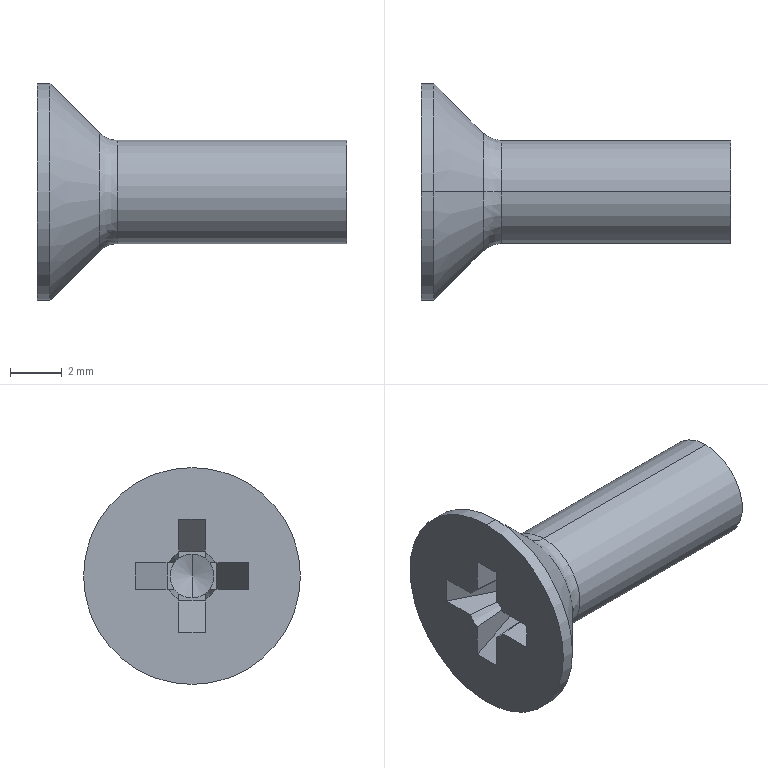Part | SolidWorks | features BaseBody 1 | 1 solid | 32 faces | box 12 x 8.4 x 8.4 mm | volume 199.797 mm3 | plane 18 | cone 8 | cylinder 4 | spline 2 | commonest cylinder face diameters 4 x2 8.4 x2
STEP:
#1=CARTESIAN_POINT('',(3.114,0.,-2.));
#2=VERTEX_POINT('',#1);
#3=CARTESIAN_POINT('',(3.114,0.,2.));
#4=VERTEX_POINT('',#3);
#5=CARTESIAN_POINT('',(3.114,0.,0.));
#6=DIRECTION('',(1.,0.,0.));
#7=DIRECTION('',(0.,0.,1.));
#8=AXIS2_PLACEMENT_3D('',#5,#6,#7);
#9=CIRCLE('',#8,2.);
#10=EDGE_CURVE('',#2,#4,#9,.T.);
#11=ORIENTED_EDGE('',*,*,#10,.F.);
#12=CARTESIAN_POINT('',(2.407,0.,-2.293));
#13=VERTEX_POINT('',#12);
#14=CARTESIAN_POINT('',(3.114,0.,-3.));
#15=DIRECTION('',(0.,-1.,0.));
#16=DIRECTION('',(0.,0.,-1.));
#17=AXIS2_PLACEMENT_3D('',#14,#15,#16);
#18=CIRCLE('',#17,1.);
#19=EDGE_CURVE('',#2,#13,#18,.T.);
#20=ORIENTED_EDGE('',*,*,#19,.T.);
#21=CARTESIAN_POINT('',(2.407,0.,2.293));
#22=VERTEX_POINT('',#21);
#23=CARTESIAN_POINT('',(2.407,0.,0.));
#24=DIRECTION('',(-1.,0.,0.));
#25=DIRECTION('',(0.,0.,1.));
#26=AXIS2_PLACEMENT_3D('',#23,#24,#25);
#27=CIRCLE('',#26,2.293);
#28=EDGE_CURVE('',#22,#13,#27,.T.);
#29=ORIENTED_EDGE('',*,*,#28,.F.);
#30=CARTESIAN_POINT('',(3.114,0.,3.));
#31=DIRECTION('',(0.,1.,0.));
#32=DIRECTION('',(0.,0.,1.));
#33=AXIS2_PLACEMENT_3D('',#30,#31,#32);
#34=CIRCLE('',#33,1.);
#35=EDGE_CURVE('',#4,#22,#34,.T.);
#36=ORIENTED_EDGE('',*,*,#35,.F.);
#37=EDGE_LOOP('',(#11,#20,#29,#36));
#38=FACE_OUTER_BOUND('',#37,.T.);
#39=CARTESIAN_POINT('',(3.114,0.,2.));
#40=CARTESIAN_POINT('',(3.114,4.,2.));
#41=CARTESIAN_POINT('',(3.114,4.,-2.));
#42=CARTESIAN_POINT('',(3.114,0.,-2.));
#43=CARTESIAN_POINT('',(2.845,0.,2.));
#44=CARTESIAN_POINT('',(2.845,4.,2.));
#45=CARTESIAN_POINT('',(2.845,4.,-2.));
#46=CARTESIAN_POINT('',(2.845,0.,-2.));
#47=CARTESIAN_POINT('',(2.597,0.,2.103));
#48=CARTESIAN_POINT('',(2.597,4.206,2.103));
#49=CARTESIAN_POINT('',(2.597,4.206,-2.103));
#50=CARTESIAN_POINT('',(2.597,0.,-2.103));
#51=CARTESIAN_POINT('',(2.407,0.,2.293));
#52=CARTESIAN_POINT('',(2.407,4.586,2.293));
#53=CARTESIAN_POINT('',(2.407,4.586,-2.293));
#54=CARTESIAN_POINT('',(2.407,0.,-2.293));
#55=(BOUNDED_SURFACE()B_SPLINE_SURFACE(3,3,((#39,#40,#41,#42),(#43,#44,#45,#46),(#47,#48,#49,#50),(#51,#52,#53,#54)),.UNSPECIFIED.,.F.,.F.,.F.)B_SPLINE_SURFACE_WITH_KNOTS((4,4),(4,4),(0.,1.),(0.,1.),.UNSPECIFIED.)GEOMETRIC_REPRESENTATION_ITEM()RATIONAL_B_SPLINE_SURFACE(((1.,0.3333,0.3333,1.),(0.9493,0.3164,0.3164,0.9493),(0.9493,0.3164,0.3164,0.9493),(1.,0.3333,0.3333,1.)))REPRESENTATION_ITEM('')SURFACE());
#56=ADVANCED_FACE('',(#38),#55,.F.);
#57=CARTESIAN_POINT('',(12.,0.,2.));
#58=VERTEX_POINT('',#57);
#59=CARTESIAN_POINT('',(12.,0.,-2.));
#60=VERTEX_POINT('',#59);
#61=CARTESIAN_POINT('',(12.,0.,0.));
#62=DIRECTION('',(-1.,0.,0.));
#63=DIRECTION('',(0.,0.,1.));
#64=AXIS2_PLACEMENT_3D('',#61,#62,#63);
#65=CIRCLE('',#64,2.);
#66=EDGE_CURVE('',#58,#60,#65,.T.);
#67=ORIENTED_EDGE('',*,*,#66,.T.);
#68=CARTESIAN_POINT('',(-6.35,0.,-2.));
#69=DIRECTION('',(-1.,0.,0.));
#70=VECTOR('',#69,1000.);
#71=LINE('',#68,#70);
#72=EDGE_CURVE('',#60,#2,#71,.T.);
#73=ORIENTED_EDGE('',*,*,#72,.T.);
#74=ORIENTED_EDGE('',*,*,#10,.T.);
#75=CARTESIAN_POINT('',(-6.35,0.,2.));
#76=DIRECTION('',(-1.,0.,0.));
#77=VECTOR('',#76,1000.);
#78=LINE('',#75,#77);
#79=EDGE_CURVE('',#58,#4,#78,.T.);
#80=ORIENTED_EDGE('',*,*,#79,.F.);
#81=EDGE_LOOP('',(#67,#73,#74,#80));
#82=FACE_OUTER_BOUND('',#81,.T.);
#83=CARTESIAN_POINT('',(-6.35,0.,0.));
#84=DIRECTION('',(-1.,0.,0.));
#85=DIRECTION('',(0.,0.,1.));
#86=AXIS2_PLACEMENT_3D('',#83,#84,#85);
#87=CYLINDRICAL_SURFACE('',#86,2.);
#88=ADVANCED_FACE('',(#82),#87,.T.);
#89=ORIENTED_EDGE('',*,*,#28,.T.);
#90=CARTESIAN_POINT('',(0.5,0.,-4.2));
#91=VERTEX_POINT('',#90);
#92=CARTESIAN_POINT('',(0.5,0.,-4.2));
#93=DIRECTION('',(-0.7071,0.,-0.7071));
#94=VECTOR('',#93,1000.);
#95=LINE('',#92,#94);
#96=EDGE_CURVE('',#13,#91,#95,.T.);
#97=ORIENTED_EDGE('',*,*,#96,.T.);
#98=CARTESIAN_POINT('',(0.5,0.,4.2));
#99=VERTEX_POINT('',#98);
#100=CARTESIAN_POINT('',(0.5,0.,0.));
#101=DIRECTION('',(1.,0.,0.));
#102=DIRECTION('',(0.,0.,1.));
#103=AXIS2_PLACEMENT_3D('',#100,#101,#102);
#104=CIRCLE('',#103,4.2);
#105=EDGE_CURVE('',#91,#99,#104,.T.);
#106=ORIENTED_EDGE('',*,*,#105,.T.);
#107=CARTESIAN_POINT('',(0.5,0.,4.2));
#108=DIRECTION('',(-0.7071,0.,0.7071));
#109=VECTOR('',#108,1000.);
#110=LINE('',#107,#109);
#111=EDGE_CURVE('',#22,#99,#110,.T.);
#112=ORIENTED_EDGE('',*,*,#111,.F.);
#113=EDGE_LOOP('',(#89,#97,#106,#112));
#114=FACE_OUTER_BOUND('',#113,.T.);
#115=CARTESIAN_POINT('',(0.5,0.,0.));
#116=DIRECTION('',(-1.,0.,0.));
#117=DIRECTION('',(0.,0.,1.));
#118=AXIS2_PLACEMENT_3D('',#115,#116,#117);
#119=CONICAL_SURFACE('',#118,4.2,0.7854);
#120=ADVANCED_FACE('',(#114),#119,.T.);
#121=ORIENTED_EDGE('',*,*,#105,.F.);
#122=CARTESIAN_POINT('',(0.,0.,-4.2));
#123=VERTEX_POINT('',#122);
#124=CARTESIAN_POINT('',(-6.35,0.,-4.2));
#125=DIRECTION('',(-1.,0.,0.));
#126=VECTOR('',#125,1000.);
#127=LINE('',#124,#126);
#128=EDGE_CURVE('',#91,#123,#127,.T.);
#129=ORIENTED_EDGE('',*,*,#128,.T.);
#130=CARTESIAN_POINT('',(0.,0.,4.2));
#131=VERTEX_POINT('',#130);
#132=CARTESIAN_POINT('',(0.,0.,0.));
#133=DIRECTION('',(1.,0.,0.));
#134=DIRECTION('',(0.,0.,1.));
#135=AXIS2_PLACEMENT_3D('',#132,#133,#134);
#136=CIRCLE('',#135,4.2);
#137=EDGE_CURVE('',#123,#131,#136,.T.);
#138=ORIENTED_EDGE('',*,*,#137,.T.);
#139=CARTESIAN_POINT('',(-6.35,0.,4.2));
#140=DIRECTION('',(-1.,0.,0.));
#141=VECTOR('',#140,1000.);
#142=LINE('',#139,#141);
#143=EDGE_CURVE('',#99,#131,#142,.T.);
#144=ORIENTED_EDGE('',*,*,#143,.F.);
#145=EDGE_LOOP('',(#121,#129,#138,#144));
#146=FACE_OUTER_BOUND('',#145,.T.);
#147=CARTESIAN_POINT('',(-6.35,0.,0.));
#148=DIRECTION('',(-1.,0.,0.));
#149=DIRECTION('',(0.,0.,1.));
#150=AXIS2_PLACEMENT_3D('',#147,#148,#149);
#151=CYLINDRICAL_SURFACE('',#150,4.2);
#152=ADVANCED_FACE('',(#146),#151,.T.);
#153=CARTESIAN_POINT('',(2.787,0.,0.));
#154=VERTEX_POINT('',#153);
#155=CARTESIAN_POINT('',(2.51,0.,0.851));
#156=VERTEX_POINT('',#155);
#157=CARTESIAN_POINT('',(2.51,0.,0.851));
#158=DIRECTION('',(-0.309,0.,0.9511));
#159=VECTOR('',#158,1000.);
#160=LINE('',#157,#159);
#161=EDGE_CURVE('',#154,#156,#160,.T.);
#162=ORIENTED_EDGE('',*,*,#161,.F.);
#163=CARTESIAN_POINT('',(2.51,0.,-0.851));
#164=VERTEX_POINT('',#163);
#165=CARTESIAN_POINT('',(2.51,0.,-0.851));
#166=DIRECTION('',(-0.309,0.,-0.9511));
#167=VECTOR('',#166,1000.);
#168=LINE('',#165,#167);
#169=EDGE_CURVE('',#154,#164,#168,.T.);
#170=ORIENTED_EDGE('',*,*,#169,.T.);
#171=CARTESIAN_POINT('',(2.51,-0.515,-0.6775));
#172=VERTEX_POINT('',#171);
#173=CARTESIAN_POINT('',(2.51,0.,0.));
#174=DIRECTION('',(1.,0.,0.));
#175=DIRECTION('',(0.,0.,1.));
#176=AXIS2_PLACEMENT_3D('',#173,#174,#175);
#177=CIRCLE('',#176,0.851);
#178=EDGE_CURVE('',#172,#164,#177,.T.);
#179=ORIENTED_EDGE('',*,*,#178,.F.);
#180=CARTESIAN_POINT('',(2.51,-0.6775,-0.515));
#181=VERTEX_POINT('',#180);
#182=CARTESIAN_POINT('',(2.51,0.,0.));
#183=DIRECTION('',(-1.,0.,0.));
#184=DIRECTION('',(0.,0.,1.));
#185=AXIS2_PLACEMENT_3D('',#182,#183,#184);
#186=CIRCLE('',#185,0.851);
#187=EDGE_CURVE('',#172,#181,#186,.T.);
#188=ORIENTED_EDGE('',*,*,#187,.T.);
#189=CARTESIAN_POINT('',(2.51,-0.6775,0.515));
#190=VERTEX_POINT('',#189);
#191=CARTESIAN_POINT('',(2.51,0.,0.));
#192=DIRECTION('',(1.,0.,0.));
#193=DIRECTION('',(0.,0.,1.));
#194=AXIS2_PLACEMENT_3D('',#191,#192,#193);
#195=CIRCLE('',#194,0.851);
#196=EDGE_CURVE('',#190,#181,#195,.T.);
#197=ORIENTED_EDGE('',*,*,#196,.F.);
#198=CARTESIAN_POINT('',(2.51,-0.515,0.6775));
#199=VERTEX_POINT('',#198);
#200=CARTESIAN_POINT('',(2.51,0.,0.));
#201=DIRECTION('',(1.,0.,0.));
#202=DIRECTION('',(0.,0.,1.));
#203=AXIS2_PLACEMENT_3D('',#200,#201,#202);
#204=CIRCLE('',#203,0.851);
#205=EDGE_CURVE('',#199,#190,#204,.T.);
#206=ORIENTED_EDGE('',*,*,#205,.F.);
#207=CARTESIAN_POINT('',(2.51,0.,0.));
#208=DIRECTION('',(1.,0.,0.));
#209=DIRECTION('',(0.,0.,1.));
#210=AXIS2_PLACEMENT_3D('',#207,#208,#209);
#211=CIRCLE('',#210,0.851);
#212=EDGE_CURVE('',#156,#199,#211,.T.);
#213=ORIENTED_EDGE('',*,*,#212,.F.);
#214=EDGE_LOOP('',(#162,#170,#179,#188,#197,#206,#213));
#215=FACE_OUTER_BOUND('',#214,.T.);
#216=CARTESIAN_POINT('',(2.51,0.,0.));
#217=DIRECTION('',(-1.,0.,0.));
#218=DIRECTION('',(0.,0.,1.));
#219=AXIS2_PLACEMENT_3D('',#216,#217,#218);
#220=CONICAL_SURFACE('',#219,0.851,1.257);
#221=ADVANCED_FACE('',(#215),#220,.F.);
#222=ORIENTED_EDGE('',*,*,#72,.F.);
#223=CARTESIAN_POINT('',(12.,0.,0.));
#224=DIRECTION('',(-1.,0.,0.));
#225=DIRECTION('',(0.,0.,1.));
#226=AXIS2_PLACEMENT_3D('',#223,#224,#225);
#227=CIRCLE('',#226,2.);
#228=EDGE_CURVE('',#60,#58,#227,.T.);
#229=ORIENTED_EDGE('',*,*,#228,.T.);
#230=ORIENTED_EDGE('',*,*,#79,.T.);
#231=CARTESIAN_POINT('',(3.114,0.,0.));
#232=DIRECTION('',(1.,0.,0.));
#233=DIRECTION('',(0.,0.,1.));
#234=AXIS2_PLACEMENT_3D('',#231,#232,#233);
#235=CIRCLE('',#234,2.);
#236=EDGE_CURVE('',#4,#2,#235,.T.);
#237=ORIENTED_EDGE('',*,*,#236,.T.);
#238=EDGE_LOOP('',(#222,#229,#230,#237));
#239=FACE_OUTER_BOUND('',#238,.T.);
#240=CARTESIAN_POINT('',(-6.35,0.,0.));
#241=DIRECTION('',(-1.,0.,0.));
#242=DIRECTION('',(0.,0.,1.));
#243=AXIS2_PLACEMENT_3D('',#240,#241,#242);
#244=CYLINDRICAL_SURFACE('',#243,2.);
#245=ADVANCED_FACE('',(#239),#244,.T.);
#246=ORIENTED_EDGE('',*,*,#19,.F.);
#247=ORIENTED_EDGE('',*,*,#236,.F.);
#248=ORIENTED_EDGE('',*,*,#35,.T.);
#249=CARTESIAN_POINT('',(2.407,0.,0.));
#250=DIRECTION('',(-1.,0.,0.));
#251=DIRECTION('',(0.,0.,1.));
#252=AXIS2_PLACEMENT_3D('',#249,#250,#251);
#253=CIRCLE('',#252,2.293);
#254=EDGE_CURVE('',#13,#22,#253,.T.);
#255=ORIENTED_EDGE('',*,*,#254,.F.);
#256=EDGE_LOOP('',(#246,#247,#248,#255));
#257=FACE_OUTER_BOUND('',#256,.T.);
#258=CARTESIAN_POINT('',(3.114,0.,-2.));
#259=CARTESIAN_POINT('',(3.114,-4.,-2.));
#260=CARTESIAN_POINT('',(3.114,-4.,2.));
#261=CARTESIAN_POINT('',(3.114,0.,2.));
#262=CARTESIAN_POINT('',(2.845,0.,-2.));
#263=CARTESIAN_POINT('',(2.845,-4.,-2.));
#264=CARTESIAN_POINT('',(2.845,-4.,2.));
#265=CARTESIAN_POINT('',(2.845,0.,2.));
#266=CARTESIAN_POINT('',(2.597,0.,-2.103));
#267=CARTESIAN_POINT('',(2.597,-4.206,-2.103));
#268=CARTESIAN_POINT('',(2.597,-4.206,2.103));
#269=CARTESIAN_POINT('',(2.597,0.,2.103));
#270=CARTESIAN_POINT('',(2.407,0.,-2.293));
#271=CARTESIAN_POINT('',(2.407,-4.586,-2.293));
#272=CARTESIAN_POINT('',(2.407,-4.586,2.293));
#273=CARTESIAN_POINT('',(2.407,0.,2.293));
#274=(BOUNDED_SURFACE()B_SPLINE_SURFACE(3,3,((#258,#259,#260,#261),(#262,#263,#264,#265),(#266,#267,#268,#269),(#270,#271,#272,#273)),.UNSPECIFIED.,.F.,.F.,.F.)B_SPLINE_SURFACE_WITH_KNOTS((4,4),(4,4),(0.,1.),(0.,1.),.UNSPECIFIED.)GEOMETRIC_REPRESENTATION_ITEM()RATIONAL_B_SPLINE_SURFACE(((1.,0.3333,0.3333,1.),(0.9493,0.3164,0.3164,0.9493),(0.9493,0.3164,0.3164,0.9493),(1.,0.3333,0.3333,1.)))REPRESENTATION_ITEM('')SURFACE());
#275=ADVANCED_FACE('',(#257),#274,.F.);
#276=ORIENTED_EDGE('',*,*,#66,.F.);
#277=ORIENTED_EDGE('',*,*,#228,.F.);
#278=EDGE_LOOP('',(#276,#277));
#279=FACE_OUTER_BOUND('',#278,.T.);
#280=CARTESIAN_POINT('',(12.,2.,0.));
#281=DIRECTION('',(1.,0.,0.));
#282=DIRECTION('',(0.,0.,-1.));
#283=AXIS2_PLACEMENT_3D('',#280,#281,#282);
#284=PLANE('',#283);
#285=ADVANCED_FACE('',(#279),#284,.T.);
#286=ORIENTED_EDGE('',*,*,#96,.F.);
#287=ORIENTED_EDGE('',*,*,#254,.T.);
#288=ORIENTED_EDGE('',*,*,#111,.T.);
#289=CARTESIAN_POINT('',(0.5,0.,0.));
#290=DIRECTION('',(1.,0.,0.));
#291=DIRECTION('',(0.,0.,1.));
#292=AXIS2_PLACEMENT_3D('',#289,#290,#291);
#293=CIRCLE('',#292,4.2);
#294=EDGE_CURVE('',#99,#91,#293,.T.);
#295=ORIENTED_EDGE('',*,*,#294,.T.);
#296=EDGE_LOOP('',(#286,#287,#288,#295));
#297=FACE_OUTER_BOUND('',#296,.T.);
#298=CARTESIAN_POINT('',(0.5,0.,0.));
#299=DIRECTION('',(-1.,0.,0.));
#300=DIRECTION('',(0.,0.,1.));
#301=AXIS2_PLACEMENT_3D('',#298,#299,#300);
#302=CONICAL_SURFACE('',#301,4.2,0.7854);
#303=ADVANCED_FACE('',(#297),#302,.T.);
#304=ORIENTED_EDGE('',*,*,#128,.F.);
#305=ORIENTED_EDGE('',*,*,#294,.F.);
#306=ORIENTED_EDGE('',*,*,#143,.T.);
#307=CARTESIAN_POINT('',(0.,0.,0.));
#308=DIRECTION('',(1.,0.,0.));
#309=DIRECTION('',(0.,0.,1.));
#310=AXIS2_PLACEMENT_3D('',#307,#308,#309);
#311=CIRCLE('',#310,4.2);
#312=EDGE_CURVE('',#131,#123,#311,.T.);
#313=ORIENTED_EDGE('',*,*,#312,.T.);
#314=EDGE_LOOP('',(#304,#305,#306,#313));
#315=FACE_OUTER_BOUND('',#314,.T.);
#316=CARTESIAN_POINT('',(-6.35,0.,0.));
#317=DIRECTION('',(-1.,0.,0.));
#318=DIRECTION('',(0.,0.,1.));
#319=AXIS2_PLACEMENT_3D('',#316,#317,#318);
#320=CYLINDRICAL_SURFACE('',#319,4.2);
#321=ADVANCED_FACE('',(#315),#320,.T.);
#322=CARTESIAN_POINT('',(0.,0.515,2.2));
#323=VERTEX_POINT('',#322);
#324=CARTESIAN_POINT('',(0.,0.515,0.888));
#325=VERTEX_POINT('',#324);
#326=CARTESIAN_POINT('',(0.,0.515,0.9486));
#327=DIRECTION('',(0.,0.,-1.));
#328=VECTOR('',#327,1000.);
#329=LINE('',#326,#328);
#330=EDGE_CURVE('',#323,#325,#329,.T.);
#331=ORIENTED_EDGE('',*,*,#330,.F.);
#332=CARTESIAN_POINT('',(0.,-0.515,2.2));
#333=VERTEX_POINT('',#332);
#334=CARTESIAN_POINT('',(0.,0.,2.2));
#335=DIRECTION('',(0.,-1.,0.));
#336=VECTOR('',#335,1000.);
#337=LINE('',#334,#336);
#338=EDGE_CURVE('',#323,#333,#337,.T.);
#339=ORIENTED_EDGE('',*,*,#338,.T.);
#340=CARTESIAN_POINT('',(0.,-0.515,0.888));
#341=VERTEX_POINT('',#340);
#342=CARTESIAN_POINT('',(0.,-0.515,-0.9486));
#343=DIRECTION('',(0.,0.,1.));
#344=VECTOR('',#343,1000.);
#345=LINE('',#342,#344);
#346=EDGE_CURVE('',#341,#333,#345,.T.);
#347=ORIENTED_EDGE('',*,*,#346,.F.);
#348=CARTESIAN_POINT('',(0.,-0.888,0.515));
#349=VERTEX_POINT('',#348);
#350=CARTESIAN_POINT('',(0.,0.,0.));
#351=DIRECTION('',(1.,0.,0.));
#352=DIRECTION('',(0.,0.,1.));
#353=AXIS2_PLACEMENT_3D('',#350,#351,#352);
#354=CIRCLE('',#353,1.027);
#355=EDGE_CURVE('',#341,#349,#354,.T.);
#356=ORIENTED_EDGE('',*,*,#355,.T.);
#357=CARTESIAN_POINT('',(0.,-2.2,0.515));
#358=VERTEX_POINT('',#357);
#359=CARTESIAN_POINT('',(0.,-0.9486,0.515));
#360=DIRECTION('',(0.,1.,0.));
#361=VECTOR('',#360,1000.);
#362=LINE('',#359,#361);
#363=EDGE_CURVE('',#358,#349,#362,.T.);
#364=ORIENTED_EDGE('',*,*,#363,.F.);
#365=CARTESIAN_POINT('',(0.,-2.2,-0.515));
#366=VERTEX_POINT('',#365);
#367=CARTESIAN_POINT('',(0.,-2.2,-0.515));
#368=DIRECTION('',(0.,0.,1.));
#369=VECTOR('',#368,1000.);
#370=LINE('',#367,#369);
#371=EDGE_CURVE('',#366,#358,#370,.T.);
#372=ORIENTED_EDGE('',*,*,#371,.F.);
#373=CARTESIAN_POINT('',(0.,-0.888,-0.515));
#374=VERTEX_POINT('',#373);
#375=CARTESIAN_POINT('',(0.,0.9486,-0.515));
#376=DIRECTION('',(0.,-1.,0.));
#377=VECTOR('',#376,1000.);
#378=LINE('',#375,#377);
#379=EDGE_CURVE('',#374,#366,#378,.T.);
#380=ORIENTED_EDGE('',*,*,#379,.F.);
#381=CARTESIAN_POINT('',(0.,-0.515,-0.888));
#382=VERTEX_POINT('',#381);
#383=CARTESIAN_POINT('',(0.,0.,0.));
#384=DIRECTION('',(1.,0.,0.));
#385=DIRECTION('',(0.,0.,1.));
#386=AXIS2_PLACEMENT_3D('',#383,#384,#385);
#387=CIRCLE('',#386,1.027);
#388=EDGE_CURVE('',#374,#382,#387,.T.);
#389=ORIENTED_EDGE('',*,*,#388,.T.);
#390=CARTESIAN_POINT('',(0.,-0.515,-2.2));
#391=VERTEX_POINT('',#390);
#392=CARTESIAN_POINT('',(0.,-0.515,-0.9486));
#393=DIRECTION('',(0.,0.,1.));
#394=VECTOR('',#393,1000.);
#395=LINE('',#392,#394);
#396=EDGE_CURVE('',#391,#382,#395,.T.);
#397=ORIENTED_EDGE('',*,*,#396,.F.);
#398=CARTESIAN_POINT('',(0.,0.515,-2.2));
#399=VERTEX_POINT('',#398);
#400=CARTESIAN_POINT('',(0.,0.515,-2.2));
#401=DIRECTION('',(0.,-1.,0.));
#402=VECTOR('',#401,1000.);
#403=LINE('',#400,#402);
#404=EDGE_CURVE('',#399,#391,#403,.T.);
#405=ORIENTED_EDGE('',*,*,#404,.F.);
#406=CARTESIAN_POINT('',(0.,0.515,-0.888));
#407=VERTEX_POINT('',#406);
#408=CARTESIAN_POINT('',(0.,0.515,0.9486));
#409=DIRECTION('',(0.,0.,-1.));
#410=VECTOR('',#409,1000.);
#411=LINE('',#408,#410);
#412=EDGE_CURVE('',#407,#399,#411,.T.);
#413=ORIENTED_EDGE('',*,*,#412,.F.);
#414=CARTESIAN_POINT('',(0.,0.888,-0.515));
#415=VERTEX_POINT('',#414);
#416=CARTESIAN_POINT('',(0.,0.,0.));
#417=DIRECTION('',(1.,0.,0.));
#418=DIRECTION('',(0.,0.,1.));
#419=AXIS2_PLACEMENT_3D('',#416,#417,#418);
#420=CIRCLE('',#419,1.027);
#421=EDGE_CURVE('',#407,#415,#420,.T.);
#422=ORIENTED_EDGE('',*,*,#421,.T.);
#423=CARTESIAN_POINT('',(0.,2.2,-0.515));
#424=VERTEX_POINT('',#423);
#425=CARTESIAN_POINT('',(0.,0.9486,-0.515));
#426=DIRECTION('',(0.,-1.,0.));
#427=VECTOR('',#426,1000.);
#428=LINE('',#425,#427);
#429=EDGE_CURVE('',#424,#415,#428,.T.);
#430=ORIENTED_EDGE('',*,*,#429,.F.);
#431=CARTESIAN_POINT('',(0.,2.2,0.515));
#432=VERTEX_POINT('',#431);
#433=CARTESIAN_POINT('',(0.,2.2,0.515));
#434=DIRECTION('',(0.,0.,-1.));
#435=VECTOR('',#434,1000.);
#436=LINE('',#433,#435);
#437=EDGE_CURVE('',#432,#424,#436,.T.);
#438=ORIENTED_EDGE('',*,*,#437,.F.);
#439=CARTESIAN_POINT('',(0.,0.888,0.515));
#440=VERTEX_POINT('',#439);
#441=CARTESIAN_POINT('',(0.,-0.9486,0.515));
#442=DIRECTION('',(0.,1.,0.));
#443=VECTOR('',#442,1000.);
#444=LINE('',#441,#443);
#445=EDGE_CURVE('',#440,#432,#444,.T.);
#446=ORIENTED_EDGE('',*,*,#445,.F.);
#447=CARTESIAN_POINT('',(0.,0.,0.));
#448=DIRECTION('',(1.,0.,0.));
#449=DIRECTION('',(0.,0.,1.));
#450=AXIS2_PLACEMENT_3D('',#447,#448,#449);
#451=CIRCLE('',#450,1.027);
#452=EDGE_CURVE('',#440,#325,#451,.T.);
#453=ORIENTED_EDGE('',*,*,#452,.T.);
#454=EDGE_LOOP('',(#331,#339,#347,#356,#364,#372,#380,#389,#397,#405,#413,#422,#430,#438,#446,#453));
#455=FACE_BOUND('',#454,.T.);
#456=ORIENTED_EDGE('',*,*,#312,.F.);
#457=ORIENTED_EDGE('',*,*,#137,.F.);
#458=EDGE_LOOP('',(#456,#457));
#459=FACE_OUTER_BOUND('',#458,.T.);
#460=CARTESIAN_POINT('',(0.,0.,0.));
#461=DIRECTION('',(-1.,0.,0.));
#462=DIRECTION('',(0.,0.,1.));
#463=AXIS2_PLACEMENT_3D('',#460,#461,#462);
#464=PLANE('',#463);
#465=ADVANCED_FACE('',(#455,#459),#464,.T.);
#466=CARTESIAN_POINT('',(2.51,0.515,0.9486));
#467=VERTEX_POINT('',#466);
#468=CARTESIAN_POINT('',(2.51,0.515,0.9486));
#469=DIRECTION('',(0.8949,0.,-0.4462));
#470=VECTOR('',#469,1000.);
#471=LINE('',#468,#470);
#472=EDGE_CURVE('',#323,#467,#471,.T.);
#473=ORIENTED_EDGE('',*,*,#472,.T.);
#474=CARTESIAN_POINT('',(2.51,-0.515,0.9486));
#475=VERTEX_POINT('',#474);
#476=CARTESIAN_POINT('',(2.51,-0.515,0.9486));
#477=DIRECTION('',(0.,-1.,0.));
#478=VECTOR('',#477,1000.);
#479=LINE('',#476,#478);
#480=EDGE_CURVE('',#467,#475,#479,.T.);
#481=ORIENTED_EDGE('',*,*,#480,.T.);
#482=CARTESIAN_POINT('',(2.51,-0.515,0.9486));
#483=DIRECTION('',(-0.8949,0.,0.4462));
#484=VECTOR('',#483,1000.);
#485=LINE('',#482,#484);
#486=EDGE_CURVE('',#475,#333,#485,.T.);
#487=ORIENTED_EDGE('',*,*,#486,.T.);
#488=ORIENTED_EDGE('',*,*,#338,.F.);
#489=EDGE_LOOP('',(#473,#481,#487,#488));
#490=FACE_OUTER_BOUND('',#489,.T.);
#491=CARTESIAN_POINT('',(2.51,-0.515,0.9486));
#492=DIRECTION('',(-0.4462,0.,-0.8949));
#493=DIRECTION('',(-0.8949,0.,0.4462));
#494=AXIS2_PLACEMENT_3D('',#491,#492,#493);
#495=PLANE('',#494);
#496=ADVANCED_FACE('',(#490),#495,.T.);
#497=CARTESIAN_POINT('',(2.51,-0.515,-0.515));
#498=DIRECTION('',(0.,0.,1.));
#499=VECTOR('',#498,1000.);
#500=LINE('',#497,#499);
#501=EDGE_CURVE('',#199,#475,#500,.T.);
#502=ORIENTED_EDGE('',*,*,#501,.T.);
#503=ORIENTED_EDGE('',*,*,#480,.F.);
#504=CARTESIAN_POINT('',(2.51,0.515,0.6775));
#505=VERTEX_POINT('',#504);
#506=CARTESIAN_POINT('',(2.51,0.515,-0.515));
#507=DIRECTION('',(0.,0.,-1.));
#508=VECTOR('',#507,1000.);
#509=LINE('',#506,#508);
#510=EDGE_CURVE('',#467,#505,#509,.T.);
#511=ORIENTED_EDGE('',*,*,#510,.T.);
#512=CARTESIAN_POINT('',(2.51,0.,0.));
#513=DIRECTION('',(1.,0.,0.));
#514=DIRECTION('',(0.,0.,1.));
#515=AXIS2_PLACEMENT_3D('',#512,#513,#514);
#516=CIRCLE('',#515,0.851);
#517=EDGE_CURVE('',#505,#156,#516,.T.);
#518=ORIENTED_EDGE('',*,*,#517,.T.);
#519=ORIENTED_EDGE('',*,*,#212,.T.);
#520=EDGE_LOOP('',(#502,#503,#511,#518,#519));
#521=FACE_OUTER_BOUND('',#520,.T.);
#522=CARTESIAN_POINT('',(2.51,-0.9486,-0.515));
#523=DIRECTION('',(-1.,0.,0.));
#524=DIRECTION('',(0.,0.,1.));
#525=AXIS2_PLACEMENT_3D('',#522,#523,#524);
#526=PLANE('',#525);
#527=ADVANCED_FACE('',(#521),#526,.T.);
#528=ORIENTED_EDGE('',*,*,#510,.F.);
#529=ORIENTED_EDGE('',*,*,#472,.F.);
#530=ORIENTED_EDGE('',*,*,#330,.T.);
#531=CARTESIAN_POINT('',(0.,0.515,0.888));
#532=CARTESIAN_POINT('',(0.6376,0.515,0.8364));
#533=CARTESIAN_POINT('',(1.275,0.515,0.7838));
#534=CARTESIAN_POINT('',(1.913,0.515,0.7293));
#535=CARTESIAN_POINT('',(2.112,0.515,0.7122));
#536=CARTESIAN_POINT('',(2.311,0.515,0.695));
#537=CARTESIAN_POINT('',(2.51,0.515,0.6775));
#538=B_SPLINE_CURVE_WITH_KNOTS('',3,(#531,#532,#533,#534,#535,#536,#537),.UNSPECIFIED.,.F.,.F.,(4,3,4),(0.,0.001919,0.002519),.UNSPECIFIED.);
#539=EDGE_CURVE('',#325,#505,#538,.T.);
#540=ORIENTED_EDGE('',*,*,#539,.T.);
#541=EDGE_LOOP('',(#528,#529,#530,#540));
#542=FACE_OUTER_BOUND('',#541,.T.);
#543=CARTESIAN_POINT('',(2.51,0.515,0.9486));
#544=DIRECTION('',(0.,-1.,0.));
#545=DIRECTION('',(0.,0.,-1.));
#546=AXIS2_PLACEMENT_3D('',#543,#544,#545);
#547=PLANE('',#546);
#548=ADVANCED_FACE('',(#542),#547,.T.);
#549=ORIENTED_EDGE('',*,*,#346,.T.);
#550=ORIENTED_EDGE('',*,*,#486,.F.);
#551=ORIENTED_EDGE('',*,*,#501,.F.);
#552=CARTESIAN_POINT('',(2.51,-0.515,0.6775));
#553=CARTESIAN_POINT('',(1.982,-0.515,0.7239));
#554=CARTESIAN_POINT('',(1.453,-0.515,0.7686));
#555=CARTESIAN_POINT('',(0.9247,-0.515,0.8124));
#556=CARTESIAN_POINT('',(0.6165,-0.515,0.8379));
#557=CARTESIAN_POINT('',(0.3083,-0.515,0.8631));
#558=CARTESIAN_POINT('',(0.,-0.515,0.888));
#559=B_SPLINE_CURVE_WITH_KNOTS('',3,(#552,#553,#554,#555,#556,#557,#558),.UNSPECIFIED.,.F.,.F.,(4,3,4),(0.,0.001591,0.002519),.UNSPECIFIED.);
#560=EDGE_CURVE('',#199,#341,#559,.T.);
#561=ORIENTED_EDGE('',*,*,#560,.T.);
#562=EDGE_LOOP('',(#549,#550,#551,#561));
#563=FACE_OUTER_BOUND('',#562,.T.);
#564=CARTESIAN_POINT('',(2.51,-0.515,-0.9486));
#565=DIRECTION('',(0.,1.,0.));
#566=DIRECTION('',(0.,0.,1.));
#567=AXIS2_PLACEMENT_3D('',#564,#565,#566);
#568=PLANE('',#567);
#569=ADVANCED_FACE('',(#563),#568,.T.);
#570=ORIENTED_EDGE('',*,*,#169,.F.);
#571=ORIENTED_EDGE('',*,*,#161,.T.);
#572=ORIENTED_EDGE('',*,*,#517,.F.);
#573=CARTESIAN_POINT('',(2.51,0.6775,0.515));
#574=VERTEX_POINT('',#573);
#575=CARTESIAN_POINT('',(2.51,0.,0.));
#576=DIRECTION('',(1.,0.,0.));
#577=DIRECTION('',(0.,0.,1.));
#578=AXIS2_PLACEMENT_3D('',#575,#576,#577);
#579=CIRCLE('',#578,0.851);
#580=EDGE_CURVE('',#574,#505,#579,.T.);
#581=ORIENTED_EDGE('',*,*,#580,.F.);
#582=CARTESIAN_POINT('',(2.51,0.6775,-0.515));
#583=VERTEX_POINT('',#582);
#584=CARTESIAN_POINT('',(2.51,0.,0.));
#585=DIRECTION('',(1.,0.,0.));
#586=DIRECTION('',(0.,0.,1.));
#587=AXIS2_PLACEMENT_3D('',#584,#585,#586);
#588=CIRCLE('',#587,0.851);
#589=EDGE_CURVE('',#583,#574,#588,.T.);
#590=ORIENTED_EDGE('',*,*,#589,.F.);
#591=CARTESIAN_POINT('',(2.51,0.515,-0.6775));
#592=VERTEX_POINT('',#591);
#593=CARTESIAN_POINT('',(2.51,0.,0.));
#594=DIRECTION('',(-1.,0.,0.));
#595=DIRECTION('',(0.,0.,1.));
#596=AXIS2_PLACEMENT_3D('',#593,#594,#595);
#597=CIRCLE('',#596,0.851);
#598=EDGE_CURVE('',#583,#592,#597,.T.);
#599=ORIENTED_EDGE('',*,*,#598,.T.);
#600=CARTESIAN_POINT('',(2.51,0.,0.));
#601=DIRECTION('',(1.,0.,0.));
#602=DIRECTION('',(0.,0.,1.));
#603=AXIS2_PLACEMENT_3D('',#600,#601,#602);
#604=CIRCLE('',#603,0.851);
#605=EDGE_CURVE('',#164,#592,#604,.T.);
#606=ORIENTED_EDGE('',*,*,#605,.F.);
#607=EDGE_LOOP('',(#570,#571,#572,#581,#590,#599,#606));
#608=FACE_OUTER_BOUND('',#607,.T.);
#609=CARTESIAN_POINT('',(2.51,0.,0.));
#610=DIRECTION('',(-1.,0.,0.));
#611=DIRECTION('',(0.,0.,1.));
#612=AXIS2_PLACEMENT_3D('',#609,#610,#611);
#613=CONICAL_SURFACE('',#612,0.851,1.257);
#614=ADVANCED_FACE('',(#608),#613,.F.);
#615=ORIENTED_EDGE('',*,*,#539,.F.);
#616=ORIENTED_EDGE('',*,*,#452,.F.);
#617=CARTESIAN_POINT('',(2.51,0.6775,0.515));
#618=CARTESIAN_POINT('',(1.982,0.7239,0.515));
#619=CARTESIAN_POINT('',(1.453,0.7686,0.515));
#620=CARTESIAN_POINT('',(0.9247,0.8124,0.515));
#621=CARTESIAN_POINT('',(0.6165,0.8379,0.515));
#622=CARTESIAN_POINT('',(0.3083,0.8631,0.515));
#623=CARTESIAN_POINT('',(0.,0.888,0.515));
#624=B_SPLINE_CURVE_WITH_KNOTS('',3,(#617,#618,#619,#620,#621,#622,#623),.UNSPECIFIED.,.F.,.F.,(4,3,4),(0.,0.001591,0.002519),.UNSPECIFIED.);
#625=EDGE_CURVE('',#574,#440,#624,.T.);
#626=ORIENTED_EDGE('',*,*,#625,.F.);
#627=ORIENTED_EDGE('',*,*,#580,.T.);
#628=EDGE_LOOP('',(#615,#616,#626,#627));
#629=FACE_OUTER_BOUND('',#628,.T.);
#630=CARTESIAN_POINT('',(0.,0.,0.));
#631=DIRECTION('',(-1.,0.,0.));
#632=DIRECTION('',(0.,0.,1.));
#633=AXIS2_PLACEMENT_3D('',#630,#631,#632);
#634=CONICAL_SURFACE('',#633,1.027,0.06981);
#635=ADVANCED_FACE('',(#629),#634,.F.);
#636=ORIENTED_EDGE('',*,*,#560,.F.);
#637=ORIENTED_EDGE('',*,*,#205,.T.);
#638=CARTESIAN_POINT('',(0.,-0.888,0.515));
#639=CARTESIAN_POINT('',(0.6376,-0.8364,0.515));
#640=CARTESIAN_POINT('',(1.275,-0.7838,0.515));
#641=CARTESIAN_POINT('',(1.913,-0.7293,0.515));
#642=CARTESIAN_POINT('',(2.112,-0.7122,0.515));
#643=CARTESIAN_POINT('',(2.311,-0.695,0.515));
#644=CARTESIAN_POINT('',(2.51,-0.6775,0.515));
#645=B_SPLINE_CURVE_WITH_KNOTS('',3,(#638,#639,#640,#641,#642,#643,#644),.UNSPECIFIED.,.F.,.F.,(4,3,4),(0.,0.001919,0.002519),.UNSPECIFIED.);
#646=EDGE_CURVE('',#349,#190,#645,.T.);
#647=ORIENTED_EDGE('',*,*,#646,.F.);
#648=ORIENTED_EDGE('',*,*,#355,.F.);
#649=EDGE_LOOP('',(#636,#637,#647,#648));
#650=FACE_OUTER_BOUND('',#649,.T.);
#651=CARTESIAN_POINT('',(0.,0.,0.));
#652=DIRECTION('',(-1.,0.,0.));
#653=DIRECTION('',(0.,0.,1.));
#654=AXIS2_PLACEMENT_3D('',#651,#652,#653);
#655=CONICAL_SURFACE('',#654,1.027,0.06981);
#656=ADVANCED_FACE('',(#650),#655,.F.);
#657=CARTESIAN_POINT('',(2.51,0.515,-0.9486));
#658=VERTEX_POINT('',#657);
#659=CARTESIAN_POINT('',(2.51,0.515,0.9486));
#660=DIRECTION('',(0.,0.,1.));
#661=VECTOR('',#660,1000.);
#662=LINE('',#659,#661);
#663=EDGE_CURVE('',#658,#592,#662,.T.);
#664=ORIENTED_EDGE('',*,*,#663,.F.);
#665=CARTESIAN_POINT('',(2.51,-0.515,-0.9486));
#666=VERTEX_POINT('',#665);
#667=CARTESIAN_POINT('',(2.51,0.515,-0.9486));
#668=DIRECTION('',(0.,1.,0.));
#669=VECTOR('',#668,1000.);
#670=LINE('',#667,#669);
#671=EDGE_CURVE('',#666,#658,#670,.T.);
#672=ORIENTED_EDGE('',*,*,#671,.F.);
#673=CARTESIAN_POINT('',(2.51,-0.515,-0.9486));
#674=DIRECTION('',(0.,0.,-1.));
#675=VECTOR('',#674,1000.);
#676=LINE('',#673,#675);
#677=EDGE_CURVE('',#172,#666,#676,.T.);
#678=ORIENTED_EDGE('',*,*,#677,.F.);
#679=ORIENTED_EDGE('',*,*,#178,.T.);
#680=ORIENTED_EDGE('',*,*,#605,.T.);
#681=EDGE_LOOP('',(#664,#672,#678,#679,#680));
#682=FACE_OUTER_BOUND('',#681,.T.);
#683=CARTESIAN_POINT('',(2.51,-0.9486,-0.515));
#684=DIRECTION('',(-1.,0.,0.));
#685=DIRECTION('',(0.,0.,1.));
#686=AXIS2_PLACEMENT_3D('',#683,#684,#685);
#687=PLANE('',#686);
#688=ADVANCED_FACE('',(#682),#687,.T.);
#689=CARTESIAN_POINT('',(2.51,-0.9486,-0.515));
#690=VERTEX_POINT('',#689);
#691=CARTESIAN_POINT('',(2.51,0.9486,-0.515));
#692=DIRECTION('',(0.,1.,0.));
#693=VECTOR('',#692,1000.);
#694=LINE('',#691,#693);
#695=EDGE_CURVE('',#690,#181,#694,.T.);
#696=ORIENTED_EDGE('',*,*,#695,.F.);
#697=CARTESIAN_POINT('',(2.51,-0.9486,0.515));
#698=VERTEX_POINT('',#697);
#699=CARTESIAN_POINT('',(2.51,-0.9486,-0.515));
#700=DIRECTION('',(0.,0.,-1.));
#701=VECTOR('',#700,1000.);
#702=LINE('',#699,#701);
#703=EDGE_CURVE('',#698,#690,#702,.T.);
#704=ORIENTED_EDGE('',*,*,#703,.F.);
#705=CARTESIAN_POINT('',(2.51,-0.9486,0.515));
#706=DIRECTION('',(0.,1.,0.));
#707=VECTOR('',#706,1000.);
#708=LINE('',#705,#707);
#709=EDGE_CURVE('',#698,#190,#708,.T.);
#710=ORIENTED_EDGE('',*,*,#709,.T.);
#711=ORIENTED_EDGE('',*,*,#196,.T.);
#712=EDGE_LOOP('',(#696,#704,#710,#711));
#713=FACE_OUTER_BOUND('',#712,.T.);
#714=CARTESIAN_POINT('',(2.51,-0.9486,-0.515));
#715=DIRECTION('',(-1.,0.,0.));
#716=DIRECTION('',(0.,0.,1.));
#717=AXIS2_PLACEMENT_3D('',#714,#715,#716);
#718=PLANE('',#717);
#719=ADVANCED_FACE('',(#713),#718,.T.);
#720=CARTESIAN_POINT('',(2.51,0.9486,0.515));
#721=VERTEX_POINT('',#720);
#722=CARTESIAN_POINT('',(2.51,-0.9486,0.515));
#723=DIRECTION('',(0.,1.,0.));
#724=VECTOR('',#723,1000.);
#725=LINE('',#722,#724);
#726=EDGE_CURVE('',#574,#721,#725,.T.);
#727=ORIENTED_EDGE('',*,*,#726,.T.);
#728=CARTESIAN_POINT('',(2.51,0.9486,-0.515));
#729=VERTEX_POINT('',#728);
#730=CARTESIAN_POINT('',(2.51,0.9486,0.515));
#731=DIRECTION('',(0.,0.,1.));
#732=VECTOR('',#731,1000.);
#733=LINE('',#730,#732);
#734=EDGE_CURVE('',#729,#721,#733,.T.);
#735=ORIENTED_EDGE('',*,*,#734,.F.);
#736=CARTESIAN_POINT('',(2.51,0.9486,-0.515));
#737=DIRECTION('',(0.,1.,0.));
#738=VECTOR('',#737,1000.);
#739=LINE('',#736,#738);
#740=EDGE_CURVE('',#583,#729,#739,.T.);
#741=ORIENTED_EDGE('',*,*,#740,.F.);
#742=ORIENTED_EDGE('',*,*,#589,.T.);
#743=EDGE_LOOP('',(#727,#735,#741,#742));
#744=FACE_OUTER_BOUND('',#743,.T.);
#745=CARTESIAN_POINT('',(2.51,-0.9486,-0.515));
#746=DIRECTION('',(-1.,0.,0.));
#747=DIRECTION('',(0.,0.,1.));
#748=AXIS2_PLACEMENT_3D('',#745,#746,#747);
#749=PLANE('',#748);
#750=ADVANCED_FACE('',(#744),#749,.T.);
#751=ORIENTED_EDGE('',*,*,#445,.T.);
#752=CARTESIAN_POINT('',(0.,2.2,0.515));
#753=DIRECTION('',(0.8949,-0.4462,0.));
#754=VECTOR('',#753,1000.);
#755=LINE('',#752,#754);
#756=EDGE_CURVE('',#432,#721,#755,.T.);
#757=ORIENTED_EDGE('',*,*,#756,.T.);
#758=ORIENTED_EDGE('',*,*,#726,.F.);
#759=ORIENTED_EDGE('',*,*,#625,.T.);
#760=EDGE_LOOP('',(#751,#757,#758,#759));
#761=FACE_OUTER_BOUND('',#760,.T.);
#762=CARTESIAN_POINT('',(2.51,-0.9486,0.515));
#763=DIRECTION('',(0.,0.,-1.));
#764=DIRECTION('',(0.,1.,0.));
#765=AXIS2_PLACEMENT_3D('',#762,#763,#764);
#766=PLANE('',#765);
#767=ADVANCED_FACE('',(#761),#766,.T.);
#768=ORIENTED_EDGE('',*,*,#709,.F.);
#769=CARTESIAN_POINT('',(2.51,-0.9486,0.515));
#770=DIRECTION('',(-0.8949,-0.4462,0.));
#771=VECTOR('',#770,1000.);
#772=LINE('',#769,#771);
#773=EDGE_CURVE('',#698,#358,#772,.T.);
#774=ORIENTED_EDGE('',*,*,#773,.T.);
#775=ORIENTED_EDGE('',*,*,#363,.T.);
#776=ORIENTED_EDGE('',*,*,#646,.T.);
#777=EDGE_LOOP('',(#768,#774,#775,#776));
#778=FACE_OUTER_BOUND('',#777,.T.);
#779=CARTESIAN_POINT('',(2.51,-0.9486,0.515));
#780=DIRECTION('',(0.,0.,-1.));
#781=DIRECTION('',(0.,1.,0.));
#782=AXIS2_PLACEMENT_3D('',#779,#780,#781);
#783=PLANE('',#782);
#784=ADVANCED_FACE('',(#778),#783,.T.);
#785=CARTESIAN_POINT('',(2.51,0.9486,-0.515));
#786=DIRECTION('',(0.8949,-0.4462,0.));
#787=VECTOR('',#786,1000.);
#788=LINE('',#785,#787);
#789=EDGE_CURVE('',#424,#729,#788,.T.);
#790=ORIENTED_EDGE('',*,*,#789,.T.);
#791=ORIENTED_EDGE('',*,*,#734,.T.);
#792=ORIENTED_EDGE('',*,*,#756,.F.);
#793=ORIENTED_EDGE('',*,*,#437,.T.);
#794=EDGE_LOOP('',(#790,#791,#792,#793));
#795=FACE_OUTER_BOUND('',#794,.T.);
#796=CARTESIAN_POINT('',(2.51,0.9486,0.515));
#797=DIRECTION('',(-0.4462,-0.8949,0.));
#798=DIRECTION('',(0.8949,-0.4462,0.));
#799=AXIS2_PLACEMENT_3D('',#796,#797,#798);
#800=PLANE('',#799);
#801=ADVANCED_FACE('',(#795),#800,.T.);
#802=ORIENTED_EDGE('',*,*,#773,.F.);
#803=ORIENTED_EDGE('',*,*,#703,.T.);
#804=CARTESIAN_POINT('',(2.51,-0.9486,-0.515));
#805=DIRECTION('',(-0.8949,-0.4462,0.));
#806=VECTOR('',#805,1000.);
#807=LINE('',#804,#806);
#808=EDGE_CURVE('',#690,#366,#807,.T.);
#809=ORIENTED_EDGE('',*,*,#808,.T.);
#810=ORIENTED_EDGE('',*,*,#371,.T.);
#811=EDGE_LOOP('',(#802,#803,#809,#810));
#812=FACE_OUTER_BOUND('',#811,.T.);
#813=CARTESIAN_POINT('',(2.51,-0.9486,-0.515));
#814=DIRECTION('',(-0.4462,0.8949,0.));
#815=DIRECTION('',(-0.8949,-0.4462,0.));
#816=AXIS2_PLACEMENT_3D('',#813,#814,#815);
#817=PLANE('',#816);
#818=ADVANCED_FACE('',(#812),#817,.T.);
#819=ORIENTED_EDGE('',*,*,#740,.T.);
#820=ORIENTED_EDGE('',*,*,#789,.F.);
#821=ORIENTED_EDGE('',*,*,#429,.T.);
#822=CARTESIAN_POINT('',(0.,0.888,-0.515));
#823=CARTESIAN_POINT('',(0.6376,0.8364,-0.515));
#824=CARTESIAN_POINT('',(1.275,0.7838,-0.515));
#825=CARTESIAN_POINT('',(1.913,0.7293,-0.515));
#826=CARTESIAN_POINT('',(2.112,0.7122,-0.515));
#827=CARTESIAN_POINT('',(2.311,0.695,-0.515));
#828=CARTESIAN_POINT('',(2.51,0.6775,-0.515));
#829=B_SPLINE_CURVE_WITH_KNOTS('',3,(#822,#823,#824,#825,#826,#827,#828),.UNSPECIFIED.,.F.,.F.,(4,3,4),(0.,0.001919,0.002519),.UNSPECIFIED.);
#830=EDGE_CURVE('',#415,#583,#829,.T.);
#831=ORIENTED_EDGE('',*,*,#830,.T.);
#832=EDGE_LOOP('',(#819,#820,#821,#831));
#833=FACE_OUTER_BOUND('',#832,.T.);
#834=CARTESIAN_POINT('',(2.51,0.9486,-0.515));
#835=DIRECTION('',(0.,0.,1.));
#836=DIRECTION('',(1.,0.,0.));
#837=AXIS2_PLACEMENT_3D('',#834,#835,#836);
#838=PLANE('',#837);
#839=ADVANCED_FACE('',(#833),#838,.T.);
#840=ORIENTED_EDGE('',*,*,#379,.T.);
#841=ORIENTED_EDGE('',*,*,#808,.F.);
#842=ORIENTED_EDGE('',*,*,#695,.T.);
#843=CARTESIAN_POINT('',(2.51,-0.6775,-0.515));
#844=CARTESIAN_POINT('',(1.982,-0.7239,-0.515));
#845=CARTESIAN_POINT('',(1.453,-0.7686,-0.515));
#846=CARTESIAN_POINT('',(0.9247,-0.8124,-0.515));
#847=CARTESIAN_POINT('',(0.6165,-0.8379,-0.515));
#848=CARTESIAN_POINT('',(0.3083,-0.8631,-0.515));
#849=CARTESIAN_POINT('',(0.,-0.888,-0.515));
#850=B_SPLINE_CURVE_WITH_KNOTS('',3,(#843,#844,#845,#846,#847,#848,#849),.UNSPECIFIED.,.F.,.F.,(4,3,4),(0.,0.001591,0.002519),.UNSPECIFIED.);
#851=EDGE_CURVE('',#181,#374,#850,.T.);
#852=ORIENTED_EDGE('',*,*,#851,.T.);
#853=EDGE_LOOP('',(#840,#841,#842,#852));
#854=FACE_OUTER_BOUND('',#853,.T.);
#855=CARTESIAN_POINT('',(2.51,0.9486,-0.515));
#856=DIRECTION('',(0.,0.,1.));
#857=DIRECTION('',(1.,0.,0.));
#858=AXIS2_PLACEMENT_3D('',#855,#856,#857);
#859=PLANE('',#858);
#860=ADVANCED_FACE('',(#854),#859,.T.);
#861=CARTESIAN_POINT('',(2.51,0.515,-0.6775));
#862=CARTESIAN_POINT('',(1.982,0.515,-0.7239));
#863=CARTESIAN_POINT('',(1.453,0.515,-0.7686));
#864=CARTESIAN_POINT('',(0.9247,0.515,-0.8124));
#865=CARTESIAN_POINT('',(0.6165,0.515,-0.8379));
#866=CARTESIAN_POINT('',(0.3083,0.515,-0.8631));
#867=CARTESIAN_POINT('',(0.,0.515,-0.888));
#868=B_SPLINE_CURVE_WITH_KNOTS('',3,(#861,#862,#863,#864,#865,#866,#867),.UNSPECIFIED.,.F.,.F.,(4,3,4),(0.,0.001591,0.002519),.UNSPECIFIED.);
#869=EDGE_CURVE('',#592,#407,#868,.T.);
#870=ORIENTED_EDGE('',*,*,#869,.F.);
#871=ORIENTED_EDGE('',*,*,#598,.F.);
#872=ORIENTED_EDGE('',*,*,#830,.F.);
#873=ORIENTED_EDGE('',*,*,#421,.F.);
#874=EDGE_LOOP('',(#870,#871,#872,#873));
#875=FACE_OUTER_BOUND('',#874,.T.);
#876=CARTESIAN_POINT('',(0.,0.,0.));
#877=DIRECTION('',(-1.,0.,0.));
#878=DIRECTION('',(0.,0.,1.));
#879=AXIS2_PLACEMENT_3D('',#876,#877,#878);
#880=CONICAL_SURFACE('',#879,1.027,0.06981);
#881=ADVANCED_FACE('',(#875),#880,.F.);
#882=CARTESIAN_POINT('',(0.,-0.515,-0.888));
#883=CARTESIAN_POINT('',(0.6376,-0.515,-0.8364));
#884=CARTESIAN_POINT('',(1.275,-0.515,-0.7838));
#885=CARTESIAN_POINT('',(1.913,-0.515,-0.7293));
#886=CARTESIAN_POINT('',(2.112,-0.515,-0.7122));
#887=CARTESIAN_POINT('',(2.311,-0.515,-0.695));
#888=CARTESIAN_POINT('',(2.51,-0.515,-0.6775));
#889=B_SPLINE_CURVE_WITH_KNOTS('',3,(#882,#883,#884,#885,#886,#887,#888),.UNSPECIFIED.,.F.,.F.,(4,3,4),(0.,0.001919,0.002519),.UNSPECIFIED.);
#890=EDGE_CURVE('',#382,#172,#889,.T.);
#891=ORIENTED_EDGE('',*,*,#890,.F.);
#892=ORIENTED_EDGE('',*,*,#388,.F.);
#893=ORIENTED_EDGE('',*,*,#851,.F.);
#894=ORIENTED_EDGE('',*,*,#187,.F.);
#895=EDGE_LOOP('',(#891,#892,#893,#894));
#896=FACE_OUTER_BOUND('',#895,.T.);
#897=CARTESIAN_POINT('',(0.,0.,0.));
#898=DIRECTION('',(-1.,0.,0.));
#899=DIRECTION('',(0.,0.,1.));
#900=AXIS2_PLACEMENT_3D('',#897,#898,#899);
#901=CONICAL_SURFACE('',#900,1.027,0.06981);
#902=ADVANCED_FACE('',(#896),#901,.F.);
#903=ORIENTED_EDGE('',*,*,#412,.T.);
#904=CARTESIAN_POINT('',(0.,0.515,-2.2));
#905=DIRECTION('',(0.8949,0.,0.4462));
#906=VECTOR('',#905,1000.);
#907=LINE('',#904,#906);
#908=EDGE_CURVE('',#399,#658,#907,.T.);
#909=ORIENTED_EDGE('',*,*,#908,.T.);
#910=ORIENTED_EDGE('',*,*,#663,.T.);
#911=ORIENTED_EDGE('',*,*,#869,.T.);
#912=EDGE_LOOP('',(#903,#909,#910,#911));
#913=FACE_OUTER_BOUND('',#912,.T.);
#914=CARTESIAN_POINT('',(2.51,0.515,0.9486));
#915=DIRECTION('',(0.,-1.,0.));
#916=DIRECTION('',(0.,0.,-1.));
#917=AXIS2_PLACEMENT_3D('',#914,#915,#916);
#918=PLANE('',#917);
#919=ADVANCED_FACE('',(#913),#918,.T.);
#920=ORIENTED_EDGE('',*,*,#677,.T.);
#921=CARTESIAN_POINT('',(2.51,-0.515,-0.9486));
#922=DIRECTION('',(-0.8949,0.,-0.4462));
#923=VECTOR('',#922,1000.);
#924=LINE('',#921,#923);
#925=EDGE_CURVE('',#666,#391,#924,.T.);
#926=ORIENTED_EDGE('',*,*,#925,.T.);
#927=ORIENTED_EDGE('',*,*,#396,.T.);
#928=ORIENTED_EDGE('',*,*,#890,.T.);
#929=EDGE_LOOP('',(#920,#926,#927,#928));
#930=FACE_OUTER_BOUND('',#929,.T.);
#931=CARTESIAN_POINT('',(2.51,-0.515,-0.9486));
#932=DIRECTION('',(0.,1.,0.));
#933=DIRECTION('',(0.,0.,1.));
#934=AXIS2_PLACEMENT_3D('',#931,#932,#933);
#935=PLANE('',#934);
#936=ADVANCED_FACE('',(#930),#935,.T.);
#937=ORIENTED_EDGE('',*,*,#925,.F.);
#938=ORIENTED_EDGE('',*,*,#671,.T.);
#939=ORIENTED_EDGE('',*,*,#908,.F.);
#940=ORIENTED_EDGE('',*,*,#404,.T.);
#941=EDGE_LOOP('',(#937,#938,#939,#940));
#942=FACE_OUTER_BOUND('',#941,.T.);
#943=CARTESIAN_POINT('',(2.51,0.515,-0.9486));
#944=DIRECTION('',(-0.4462,0.,0.8949));
#945=DIRECTION('',(0.8949,0.,0.4462));
#946=AXIS2_PLACEMENT_3D('',#943,#944,#945);
#947=PLANE('',#946);
#948=ADVANCED_FACE('',(#942),#947,.T.);
#949=CLOSED_SHELL('',(#56,#88,#120,#152,#221,#245,#275,#285,#303,#321,#465,#496,#527,#548,#569,#614,#635,#656,#688,#719,#750,#767,#784,#801,#818,#839,#860,#881,#902,#919,#936,#948));
#950=MANIFOLD_SOLID_BREP('',#949);
#951=CARTESIAN_POINT('',(0.,0.,0.));
#952=DIRECTION('',(0.,0.,1.));
#953=DIRECTION('',(1.,0.,0.));
#954=AXIS2_PLACEMENT_3D('',#951,#952,#953);
#955=(LENGTH_UNIT()NAMED_UNIT(*)SI_UNIT(.MILLI.,.METRE.));
#956=UNCERTAINTY_MEASURE_WITH_UNIT(LENGTH_MEASURE(0.00001),#955,'','');
#957=(NAMED_UNIT(*)PLANE_ANGLE_UNIT()SI_UNIT($,.RADIAN.));
#958=(NAMED_UNIT(*)SI_UNIT($,.STERADIAN.)SOLID_ANGLE_UNIT());
#959=(GEOMETRIC_REPRESENTATION_CONTEXT(3)GLOBAL_UNCERTAINTY_ASSIGNED_CONTEXT((#956))GLOBAL_UNIT_ASSIGNED_CONTEXT((#955,#957,#958))REPRESENTATION_CONTEXT('',''));
#960=ADVANCED_BREP_SHAPE_REPRESENTATION('',(#950,#954),#959);